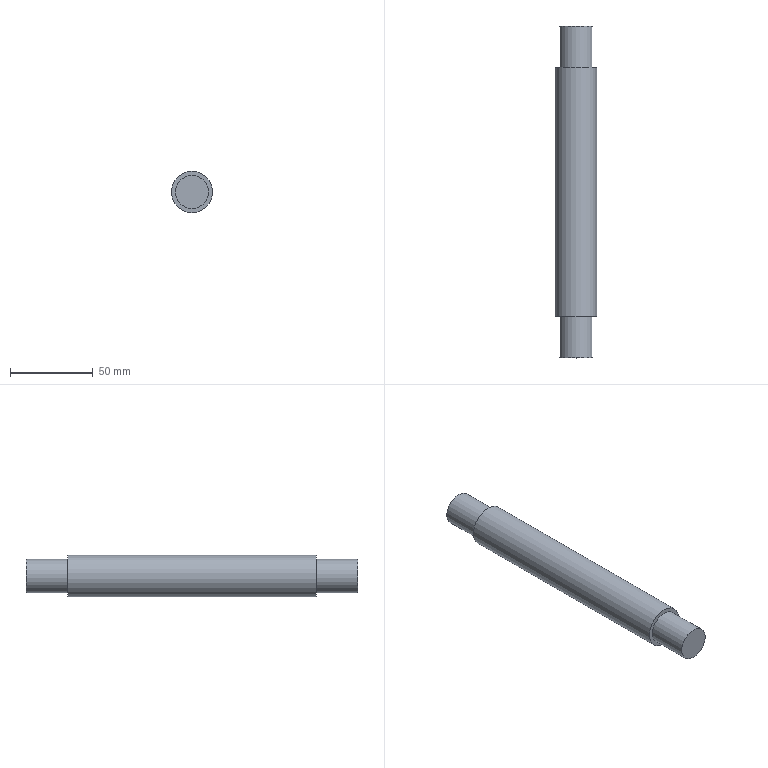Part | STEP file | 冲床-300配套压波_id822_x_t | 1 solid | 7 faces | box 25 x 200 x 25 mm | volume 89339 mm3 | plane 4 | cylinder 3 | commonest cylinder face diameters 20 x2 25 x1
STEP:
#1=CARTESIAN_POINT('',(1620.,100.,142.5));
#2=VERTEX_POINT('',#1);
#3=CARTESIAN_POINT('',(1620.,100.,132.5));
#4=DIRECTION('',(0.,1.,0.));
#5=DIRECTION('',(0.,0.,1.));
#6=AXIS2_PLACEMENT_3D('',#3,#4,#5);
#7=CIRCLE('',#6,10.);
#8=EDGE_CURVE('',#2,#2,#7,.T.);
#9=ORIENTED_EDGE('',*,*,#8,.T.);
#10=EDGE_LOOP('',(#9));
#11=FACE_OUTER_BOUND('',#10,.T.);
#12=CARTESIAN_POINT('',(1620.,100.,132.5));
#13=DIRECTION('',(0.,1.,0.));
#14=DIRECTION('',(0.,0.,-1.));
#15=AXIS2_PLACEMENT_3D('',#12,#13,#14);
#16=PLANE('',#15);
#17=ADVANCED_FACE('',(#11),#16,.T.);
#18=CARTESIAN_POINT('',(1620.,75.,142.5));
#19=VERTEX_POINT('',#18);
#20=CARTESIAN_POINT('',(1620.,75.,132.5));
#21=DIRECTION('',(0.,1.,0.));
#22=DIRECTION('',(0.,0.,1.));
#23=AXIS2_PLACEMENT_3D('',#20,#21,#22);
#24=CIRCLE('',#23,10.);
#25=EDGE_CURVE('',#19,#19,#24,.T.);
#26=ORIENTED_EDGE('',*,*,#25,.T.);
#27=EDGE_LOOP('',(#26));
#28=FACE_BOUND('',#27,.T.);
#29=ORIENTED_EDGE('',*,*,#8,.F.);
#30=EDGE_LOOP('',(#29));
#31=FACE_BOUND('',#30,.T.);
#32=CARTESIAN_POINT('',(1620.,75.,132.5));
#33=DIRECTION('',(0.,1.,0.));
#34=DIRECTION('',(0.,0.,-1.));
#35=AXIS2_PLACEMENT_3D('',#32,#33,#34);
#36=CYLINDRICAL_SURFACE('',#35,10.);
#37=ADVANCED_FACE('',(#28,#31),#36,.T.);
#38=ORIENTED_EDGE('',*,*,#25,.F.);
#39=EDGE_LOOP('',(#38));
#40=FACE_BOUND('',#39,.T.);
#41=CARTESIAN_POINT('',(1620.,75.,145.));
#42=VERTEX_POINT('',#41);
#43=CARTESIAN_POINT('',(1620.,75.,132.5));
#44=DIRECTION('',(0.,1.,0.));
#45=DIRECTION('',(0.,0.,1.));
#46=AXIS2_PLACEMENT_3D('',#43,#44,#45);
#47=CIRCLE('',#46,12.5);
#48=EDGE_CURVE('',#42,#42,#47,.T.);
#49=ORIENTED_EDGE('',*,*,#48,.T.);
#50=EDGE_LOOP('',(#49));
#51=FACE_BOUND('',#50,.T.);
#52=CARTESIAN_POINT('',(1620.,75.,132.5));
#53=DIRECTION('',(0.,1.,0.));
#54=DIRECTION('',(0.,0.,-1.));
#55=AXIS2_PLACEMENT_3D('',#52,#53,#54);
#56=PLANE('',#55);
#57=ADVANCED_FACE('',(#40,#51),#56,.T.);
#58=CARTESIAN_POINT('',(1620.,-100.,122.5));
#59=VERTEX_POINT('',#58);
#60=CARTESIAN_POINT('',(1620.,-100.,132.5));
#61=DIRECTION('',(0.,-1.,0.));
#62=DIRECTION('',(0.,0.,-1.));
#63=AXIS2_PLACEMENT_3D('',#60,#61,#62);
#64=CIRCLE('',#63,10.);
#65=EDGE_CURVE('',#59,#59,#64,.T.);
#66=ORIENTED_EDGE('',*,*,#65,.T.);
#67=EDGE_LOOP('',(#66));
#68=FACE_OUTER_BOUND('',#67,.T.);
#69=CARTESIAN_POINT('',(2025.,-100.,-25.));
#70=DIRECTION('',(0.,-1.,0.));
#71=DIRECTION('',(0.,0.,-1.));
#72=AXIS2_PLACEMENT_3D('',#69,#70,#71);
#73=PLANE('',#72);
#74=ADVANCED_FACE('',(#68),#73,.T.);
#75=ORIENTED_EDGE('',*,*,#65,.F.);
#76=EDGE_LOOP('',(#75));
#77=FACE_BOUND('',#76,.T.);
#78=CARTESIAN_POINT('',(1620.,-75.,142.5));
#79=VERTEX_POINT('',#78);
#80=CARTESIAN_POINT('',(1620.,-75.,132.5));
#81=DIRECTION('',(0.,-1.,0.));
#82=DIRECTION('',(0.,0.,1.));
#83=AXIS2_PLACEMENT_3D('',#80,#81,#82);
#84=CIRCLE('',#83,10.);
#85=EDGE_CURVE('',#79,#79,#84,.T.);
#86=ORIENTED_EDGE('',*,*,#85,.T.);
#87=EDGE_LOOP('',(#86));
#88=FACE_BOUND('',#87,.T.);
#89=CARTESIAN_POINT('',(1620.,-70.,132.5));
#90=DIRECTION('',(0.,-1.,0.));
#91=DIRECTION('',(0.,0.,-1.));
#92=AXIS2_PLACEMENT_3D('',#89,#90,#91);
#93=CYLINDRICAL_SURFACE('',#92,10.);
#94=ADVANCED_FACE('',(#77,#88),#93,.T.);
#95=ORIENTED_EDGE('',*,*,#85,.F.);
#96=EDGE_LOOP('',(#95));
#97=FACE_BOUND('',#96,.T.);
#98=CARTESIAN_POINT('',(1620.,-75.,145.));
#99=VERTEX_POINT('',#98);
#100=CARTESIAN_POINT('',(1620.,-75.,132.5));
#101=DIRECTION('',(0.,1.,0.));
#102=DIRECTION('',(0.,0.,1.));
#103=AXIS2_PLACEMENT_3D('',#100,#101,#102);
#104=CIRCLE('',#103,12.5);
#105=EDGE_CURVE('',#99,#99,#104,.T.);
#106=ORIENTED_EDGE('',*,*,#105,.F.);
#107=EDGE_LOOP('',(#106));
#108=FACE_BOUND('',#107,.T.);
#109=CARTESIAN_POINT('',(1620.,-75.,132.5));
#110=DIRECTION('',(0.,1.,0.));
#111=DIRECTION('',(0.,0.,1.));
#112=AXIS2_PLACEMENT_3D('',#109,#110,#111);
#113=PLANE('',#112);
#114=ADVANCED_FACE('',(#97,#108),#113,.F.);
#115=ORIENTED_EDGE('',*,*,#105,.T.);
#116=EDGE_LOOP('',(#115));
#117=FACE_BOUND('',#116,.T.);
#118=ORIENTED_EDGE('',*,*,#48,.F.);
#119=EDGE_LOOP('',(#118));
#120=FACE_BOUND('',#119,.T.);
#121=CARTESIAN_POINT('',(1620.,-75.,132.5));
#122=DIRECTION('',(0.,1.,0.));
#123=DIRECTION('',(0.,0.,1.));
#124=AXIS2_PLACEMENT_3D('',#121,#122,#123);
#125=CYLINDRICAL_SURFACE('',#124,12.5);
#126=ADVANCED_FACE('',(#117,#120),#125,.T.);
#127=CLOSED_SHELL('',(#17,#37,#57,#74,#94,#114,#126));
#128=MANIFOLD_SOLID_BREP('',#127);
#129=(LENGTH_UNIT()NAMED_UNIT(*)SI_UNIT(.MILLI.,.METRE.));
#130=UNCERTAINTY_MEASURE_WITH_UNIT(LENGTH_MEASURE(0.00002),#129,'','');
#131=(NAMED_UNIT(*)PLANE_ANGLE_UNIT()SI_UNIT($,.RADIAN.));
#132=PLANE_ANGLE_MEASURE_WITH_UNIT(PLANE_ANGLE_MEASURE(0.01745),#131);
#133=DIMENSIONAL_EXPONENTS(0.,0.,0.,0.,0.,0.,0.);
#134=(CONVERSION_BASED_UNIT('DEGREE',#132)NAMED_UNIT(#133)PLANE_ANGLE_UNIT());
#135=(NAMED_UNIT(*)SI_UNIT($,.STERADIAN.)SOLID_ANGLE_UNIT());
#136=(GEOMETRIC_REPRESENTATION_CONTEXT(3)GLOBAL_UNCERTAINTY_ASSIGNED_CONTEXT((#130))GLOBAL_UNIT_ASSIGNED_CONTEXT((#129,#134,#135))REPRESENTATION_CONTEXT('',''));
#137=ADVANCED_BREP_SHAPE_REPRESENTATION('',(#128),#136);